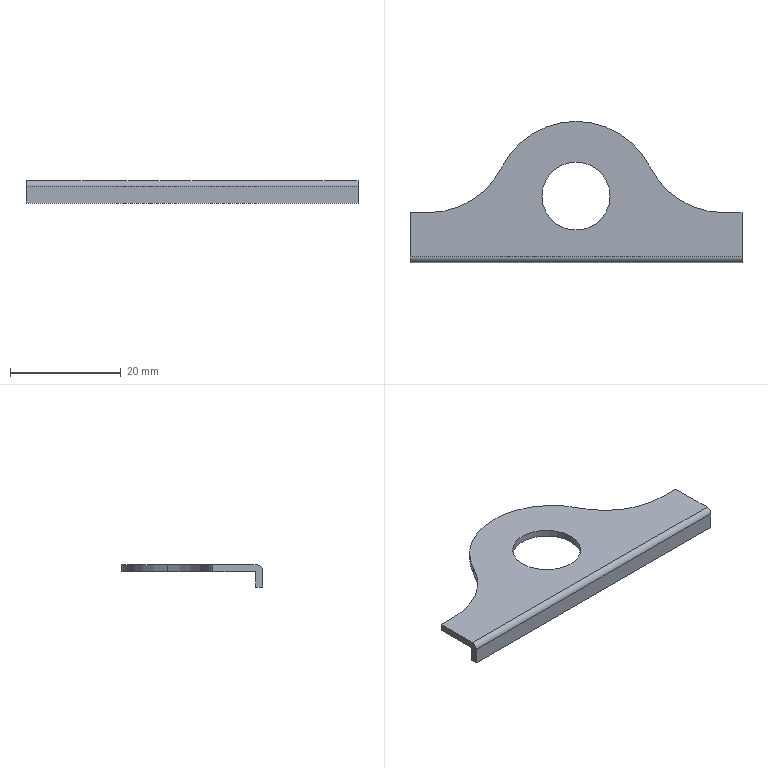Part | STEP file | gslz 2016.10.28-13_id962_x_t | 1 solid | 14 faces | box 60 x 25.5 x 4 mm | volume 1272 mm3 | plane 9 | cylinder 5 | commonest cylinder face diameters 30 x3 2 x1 12.3 x1
STEP:
#1=CARTESIAN_POINT('',(0.,0.,0.));
#2=DIRECTION('',(0.,0.,1.));
#3=DIRECTION('',(1.,0.,0.));
#4=AXIS2_PLACEMENT_3D('',#1,#2,#3);
#5=CARTESIAN_POINT('',(-668.704,-254.,1.25));
#6=VERTEX_POINT('',#5);
#7=CARTESIAN_POINT('',(-662.554,-254.,1.25));
#8=DIRECTION('',(0.,0.,1.));
#9=DIRECTION('',(-1.,0.,0.));
#10=AXIS2_PLACEMENT_3D('',#7,#8,#9);
#11=CIRCLE('',#10,6.15);
#12=CARTESIAN_POINT('',(1793.591,319.067,1.25));
#13=DIRECTION('',(0.,0.,1.));
#14=DIRECTION('',(1.,0.,0.));
#15=AXIS2_PLACEMENT_3D('',#12,#13,#14);
#16=PLANE('',#15);
#17=CARTESIAN_POINT('',(-2456.145,-573.067));
#18=DIRECTION('',(-1.,0.));
#19=AXIS2_PLACEMENT_2D('',#17,#18);
#20=CIRCLE('',#19,6.15);
#21=(GEOMETRIC_REPRESENTATION_CONTEXT(2)PARAMETRIC_REPRESENTATION_CONTEXT()REPRESENTATION_CONTEXT('',''));
#22=DEFINITIONAL_REPRESENTATION('',(#20),#21);
#23=PCURVE('',#16,#22);
#24=CARTESIAN_POINT('',(-662.554,-254.,2.5));
#25=DIRECTION('',(0.,0.,-1.));
#26=DIRECTION('',(1.,0.,0.));
#27=AXIS2_PLACEMENT_3D('',#24,#25,#26);
#28=CYLINDRICAL_SURFACE('',#27,6.15);
#29=CARTESIAN_POINT('',(9.425,1.25));
#30=DIRECTION('',(-1.,0.));
#31=VECTOR('',#30,1.);
#32=LINE('',#29,#31);
#33=(GEOMETRIC_REPRESENTATION_CONTEXT(2)PARAMETRIC_REPRESENTATION_CONTEXT()REPRESENTATION_CONTEXT('',''));
#34=DEFINITIONAL_REPRESENTATION('',(#32),#33);
#35=PCURVE('',#28,#34);
#36=SURFACE_CURVE('',#11,(#23,#35),.PCURVE_S1.);
#37=EDGE_CURVE('',#6,#6,#36,.T.);
#38=ORIENTED_EDGE('',*,*,#37,.F.);
#39=EDGE_LOOP('',(#38));
#40=FACE_BOUND('',#39,.T.);
#41=CARTESIAN_POINT('',(-692.554,-257.,1.25));
#42=VERTEX_POINT('',#41);
#43=CARTESIAN_POINT('',(-689.345,-257.,1.25));
#44=VERTEX_POINT('',#43);
#45=CARTESIAN_POINT('',(1793.591,-257.,1.25));
#46=DIRECTION('',(1.,0.,0.));
#47=VECTOR('',#46,1.);
#48=LINE('',#45,#47);
#49=CARTESIAN_POINT('',(0.,-576.067));
#50=DIRECTION('',(1.,0.));
#51=VECTOR('',#50,1.);
#52=LINE('',#49,#51);
#53=(GEOMETRIC_REPRESENTATION_CONTEXT(2)PARAMETRIC_REPRESENTATION_CONTEXT()REPRESENTATION_CONTEXT('',''));
#54=DEFINITIONAL_REPRESENTATION('',(#52),#53);
#55=PCURVE('',#16,#54);
#56=CARTESIAN_POINT('',(-705.557,-257.,2.5));
#57=DIRECTION('',(0.,1.,0.));
#58=DIRECTION('',(0.,0.,1.));
#59=AXIS2_PLACEMENT_3D('',#56,#57,#58);
#60=PLANE('',#59);
#61=CARTESIAN_POINT('',(-1.25,2499.149));
#62=DIRECTION('',(0.,1.));
#63=VECTOR('',#62,1.);
#64=LINE('',#61,#63);
#65=(GEOMETRIC_REPRESENTATION_CONTEXT(2)PARAMETRIC_REPRESENTATION_CONTEXT()REPRESENTATION_CONTEXT('',''));
#66=DEFINITIONAL_REPRESENTATION('',(#64),#65);
#67=PCURVE('',#60,#66);
#68=SURFACE_CURVE('',#48,(#55,#67),.PCURVE_S1.);
#69=EDGE_CURVE('',#42,#44,#68,.T.);
#70=ORIENTED_EDGE('',*,*,#69,.F.);
#71=CARTESIAN_POINT('',(-692.554,-265.,1.25));
#72=VERTEX_POINT('',#71);
#73=CARTESIAN_POINT('',(-692.554,319.067,1.25));
#74=DIRECTION('',(0.,1.,0.));
#75=VECTOR('',#74,1.);
#76=LINE('',#73,#75);
#77=CARTESIAN_POINT('',(-2486.145,0.));
#78=DIRECTION('',(0.,1.));
#79=VECTOR('',#78,1.);
#80=LINE('',#77,#79);
#81=(GEOMETRIC_REPRESENTATION_CONTEXT(2)PARAMETRIC_REPRESENTATION_CONTEXT()REPRESENTATION_CONTEXT('',''));
#82=DEFINITIONAL_REPRESENTATION('',(#80),#81);
#83=PCURVE('',#16,#82);
#84=CARTESIAN_POINT('',(-692.554,-244.358,-2.25));
#85=DIRECTION('',(-1.,0.,0.));
#86=DIRECTION('',(0.,0.,1.));
#87=AXIS2_PLACEMENT_3D('',#84,#85,#86);
#88=PLANE('',#87);
#89=CARTESIAN_POINT('',(3.5,563.425));
#90=DIRECTION('',(0.,1.));
#91=VECTOR('',#90,1.);
#92=LINE('',#89,#91);
#93=(GEOMETRIC_REPRESENTATION_CONTEXT(2)PARAMETRIC_REPRESENTATION_CONTEXT()REPRESENTATION_CONTEXT('',''));
#94=DEFINITIONAL_REPRESENTATION('',(#92),#93);
#95=PCURVE('',#88,#94);
#96=SURFACE_CURVE('',#76,(#83,#95),.PCURVE_S1.);
#97=EDGE_CURVE('',#72,#42,#96,.T.);
#98=ORIENTED_EDGE('',*,*,#97,.F.);
#99=CARTESIAN_POINT('',(-632.554,-265.,1.25));
#100=VERTEX_POINT('',#99);
#101=CARTESIAN_POINT('',(1793.591,-265.,1.25));
#102=DIRECTION('',(1.,0.,0.));
#103=VECTOR('',#102,1.);
#104=LINE('',#101,#103);
#105=CARTESIAN_POINT('',(0.,-584.067));
#106=DIRECTION('',(1.,0.));
#107=VECTOR('',#106,1.);
#108=LINE('',#105,#107);
#109=(GEOMETRIC_REPRESENTATION_CONTEXT(2)PARAMETRIC_REPRESENTATION_CONTEXT()REPRESENTATION_CONTEXT('',''));
#110=DEFINITIONAL_REPRESENTATION('',(#108),#109);
#111=PCURVE('',#16,#110);
#112=CARTESIAN_POINT('',(1793.591,-265.,0.25));
#113=DIRECTION('',(1.,0.,0.));
#114=DIRECTION('',(0.,1.,0.));
#115=AXIS2_PLACEMENT_3D('',#112,#113,#114);
#116=CYLINDRICAL_SURFACE('',#115,1.);
#117=CARTESIAN_POINT('',(1.571,0.));
#118=DIRECTION('',(0.,1.));
#119=VECTOR('',#118,1.);
#120=LINE('',#117,#119);
#121=(GEOMETRIC_REPRESENTATION_CONTEXT(2)PARAMETRIC_REPRESENTATION_CONTEXT()REPRESENTATION_CONTEXT('',''));
#122=DEFINITIONAL_REPRESENTATION('',(#120),#121);
#123=PCURVE('',#116,#122);
#124=SURFACE_CURVE('',#104,(#111,#123),.PCURVE_S1.);
#125=EDGE_CURVE('',#72,#100,#124,.T.);
#126=ORIENTED_EDGE('',*,*,#125,.T.);
#127=CARTESIAN_POINT('',(-632.554,-257.,1.25));
#128=VERTEX_POINT('',#127);
#129=CARTESIAN_POINT('',(-632.554,319.067,1.25));
#130=DIRECTION('',(0.,1.,0.));
#131=VECTOR('',#130,1.);
#132=LINE('',#129,#131);
#133=CARTESIAN_POINT('',(-2426.145,0.));
#134=DIRECTION('',(0.,1.));
#135=VECTOR('',#134,1.);
#136=LINE('',#133,#135);
#137=(GEOMETRIC_REPRESENTATION_CONTEXT(2)PARAMETRIC_REPRESENTATION_CONTEXT()REPRESENTATION_CONTEXT('',''));
#138=DEFINITIONAL_REPRESENTATION('',(#136),#137);
#139=PCURVE('',#16,#138);
#140=CARTESIAN_POINT('',(-632.554,-244.358,-2.25));
#141=DIRECTION('',(1.,0.,0.));
#142=DIRECTION('',(0.,0.,-1.));
#143=AXIS2_PLACEMENT_3D('',#140,#141,#142);
#144=PLANE('',#143);
#145=CARTESIAN_POINT('',(-3.5,563.425));
#146=DIRECTION('',(0.,1.));
#147=VECTOR('',#146,1.);
#148=LINE('',#145,#147);
#149=(GEOMETRIC_REPRESENTATION_CONTEXT(2)PARAMETRIC_REPRESENTATION_CONTEXT()REPRESENTATION_CONTEXT('',''));
#150=DEFINITIONAL_REPRESENTATION('',(#148),#149);
#151=PCURVE('',#144,#150);
#152=SURFACE_CURVE('',#132,(#139,#151),.PCURVE_S1.);
#153=EDGE_CURVE('',#100,#128,#152,.T.);
#154=ORIENTED_EDGE('',*,*,#153,.T.);
#155=CARTESIAN_POINT('',(-635.763,-257.,1.25));
#156=VERTEX_POINT('',#155);
#157=CARTESIAN_POINT('',(-2874.517,-257.,1.25));
#158=DIRECTION('',(1.,0.,0.));
#159=VECTOR('',#158,1.);
#160=LINE('',#157,#159);
#161=CARTESIAN_POINT('',(-4668.108,-576.067));
#162=DIRECTION('',(1.,0.));
#163=VECTOR('',#162,1.);
#164=LINE('',#161,#163);
#165=(GEOMETRIC_REPRESENTATION_CONTEXT(2)PARAMETRIC_REPRESENTATION_CONTEXT()REPRESENTATION_CONTEXT('',''));
#166=DEFINITIONAL_REPRESENTATION('',(#164),#165);
#167=PCURVE('',#16,#166);
#168=CARTESIAN_POINT('',(-614.757,-257.,2.5));
#169=DIRECTION('',(0.,1.,0.));
#170=DIRECTION('',(-1.,0.,0.));
#171=AXIS2_PLACEMENT_3D('',#168,#169,#170);
#172=PLANE('',#171);
#173=CARTESIAN_POINT('',(2259.76,-1.25));
#174=DIRECTION('',(-1.,0.));
#175=VECTOR('',#174,1.);
#176=LINE('',#173,#175);
#177=(GEOMETRIC_REPRESENTATION_CONTEXT(2)PARAMETRIC_REPRESENTATION_CONTEXT()REPRESENTATION_CONTEXT('',''));
#178=DEFINITIONAL_REPRESENTATION('',(#176),#177);
#179=PCURVE('',#172,#178);
#180=SURFACE_CURVE('',#160,(#167,#179),.PCURVE_S1.);
#181=EDGE_CURVE('',#156,#128,#180,.T.);
#182=ORIENTED_EDGE('',*,*,#181,.F.);
#183=CARTESIAN_POINT('',(-649.158,-248.75,1.25));
#184=VERTEX_POINT('',#183);
#185=CARTESIAN_POINT('',(-635.763,-242.,1.25));
#186=DIRECTION('',(0.,0.,-1.));
#187=DIRECTION('',(-1.,0.,0.));
#188=AXIS2_PLACEMENT_3D('',#185,#186,#187);
#189=CIRCLE('',#188,15.);
#190=CARTESIAN_POINT('',(-2444.354,-561.067));
#191=CARTESIAN_POINT('',(-2444.354,-535.086));
#192=CARTESIAN_POINT('',(-2421.854,-548.076));
#193=CARTESIAN_POINT('',(-2399.354,-561.067));
#194=CARTESIAN_POINT('',(-2421.854,-574.057));
#195=CARTESIAN_POINT('',(-2444.354,-587.048));
#196=CARTESIAN_POINT('',(-2444.354,-561.067));
#197=(BOUNDED_CURVE()B_SPLINE_CURVE(2,(#190,#191,#192,#193,#194,#195,#196),.UNSPECIFIED.,.T.,.F.)B_SPLINE_CURVE_WITH_KNOTS((1,2,2,2,2,1),(-2.094,0.,2.094,4.189,6.283,8.378),.UNSPECIFIED.)CURVE()GEOMETRIC_REPRESENTATION_ITEM()RATIONAL_B_SPLINE_CURVE((1.,0.5,1.,0.5,1.,0.5,1.))REPRESENTATION_ITEM(''));
#198=(GEOMETRIC_REPRESENTATION_CONTEXT(2)PARAMETRIC_REPRESENTATION_CONTEXT()REPRESENTATION_CONTEXT('',''));
#199=DEFINITIONAL_REPRESENTATION('',(#197),#198);
#200=PCURVE('',#16,#199);
#201=CARTESIAN_POINT('',(-635.763,-242.,2.5));
#202=DIRECTION('',(0.,0.,-1.));
#203=DIRECTION('',(1.,0.,0.));
#204=AXIS2_PLACEMENT_3D('',#201,#202,#203);
#205=CYLINDRICAL_SURFACE('',#204,15.);
#206=CARTESIAN_POINT('',(-3.142,1.25));
#207=DIRECTION('',(1.,0.));
#208=VECTOR('',#207,1.);
#209=LINE('',#206,#208);
#210=(GEOMETRIC_REPRESENTATION_CONTEXT(2)PARAMETRIC_REPRESENTATION_CONTEXT()REPRESENTATION_CONTEXT('',''));
#211=DEFINITIONAL_REPRESENTATION('',(#209),#210);
#212=PCURVE('',#205,#211);
#213=SURFACE_CURVE('',#189,(#200,#212),.PCURVE_S1.);
#214=EDGE_CURVE('',#156,#184,#213,.T.);
#215=ORIENTED_EDGE('',*,*,#214,.T.);
#216=CARTESIAN_POINT('',(-675.949,-248.75,1.25));
#217=VERTEX_POINT('',#216);
#218=CARTESIAN_POINT('',(-662.554,-255.5,1.25));
#219=DIRECTION('',(0.,0.,1.));
#220=DIRECTION('',(-1.,0.,0.));
#221=AXIS2_PLACEMENT_3D('',#218,#219,#220);
#222=CIRCLE('',#221,15.);
#223=CARTESIAN_POINT('',(-2456.145,-574.567));
#224=DIRECTION('',(-1.,0.));
#225=AXIS2_PLACEMENT_2D('',#223,#224);
#226=CIRCLE('',#225,15.);
#227=(GEOMETRIC_REPRESENTATION_CONTEXT(2)PARAMETRIC_REPRESENTATION_CONTEXT()REPRESENTATION_CONTEXT('',''));
#228=DEFINITIONAL_REPRESENTATION('',(#226),#227);
#229=PCURVE('',#16,#228);
#230=CARTESIAN_POINT('',(-662.554,-255.5,2.5));
#231=DIRECTION('',(0.,0.,-1.));
#232=DIRECTION('',(1.,0.,0.));
#233=AXIS2_PLACEMENT_3D('',#230,#231,#232);
#234=CYLINDRICAL_SURFACE('',#233,15.);
#235=CARTESIAN_POINT('',(9.425,1.25));
#236=DIRECTION('',(-1.,0.));
#237=VECTOR('',#236,1.);
#238=LINE('',#235,#237);
#239=(GEOMETRIC_REPRESENTATION_CONTEXT(2)PARAMETRIC_REPRESENTATION_CONTEXT()REPRESENTATION_CONTEXT('',''));
#240=DEFINITIONAL_REPRESENTATION('',(#238),#239);
#241=PCURVE('',#234,#240);
#242=SURFACE_CURVE('',#222,(#229,#241),.PCURVE_S1.);
#243=EDGE_CURVE('',#184,#217,#242,.T.);
#244=ORIENTED_EDGE('',*,*,#243,.T.);
#245=CARTESIAN_POINT('',(-689.345,-242.,1.25));
#246=DIRECTION('',(0.,0.,-1.));
#247=DIRECTION('',(-1.,0.,0.));
#248=AXIS2_PLACEMENT_3D('',#245,#246,#247);
#249=CIRCLE('',#248,15.);
#250=CARTESIAN_POINT('',(-2497.936,-561.067));
#251=CARTESIAN_POINT('',(-2497.936,-535.086));
#252=CARTESIAN_POINT('',(-2475.436,-548.076));
#253=CARTESIAN_POINT('',(-2452.936,-561.067));
#254=CARTESIAN_POINT('',(-2475.436,-574.057));
#255=CARTESIAN_POINT('',(-2497.936,-587.048));
#256=CARTESIAN_POINT('',(-2497.936,-561.067));
#257=(BOUNDED_CURVE()B_SPLINE_CURVE(2,(#250,#251,#252,#253,#254,#255,#256),.UNSPECIFIED.,.T.,.F.)B_SPLINE_CURVE_WITH_KNOTS((1,2,2,2,2,1),(-2.094,0.,2.094,4.189,6.283,8.378),.UNSPECIFIED.)CURVE()GEOMETRIC_REPRESENTATION_ITEM()RATIONAL_B_SPLINE_CURVE((1.,0.5,1.,0.5,1.,0.5,1.))REPRESENTATION_ITEM(''));
#258=(GEOMETRIC_REPRESENTATION_CONTEXT(2)PARAMETRIC_REPRESENTATION_CONTEXT()REPRESENTATION_CONTEXT('',''));
#259=DEFINITIONAL_REPRESENTATION('',(#257),#258);
#260=PCURVE('',#16,#259);
#261=CARTESIAN_POINT('',(-689.345,-242.,2.5));
#262=DIRECTION('',(0.,0.,-1.));
#263=DIRECTION('',(1.,0.,0.));
#264=AXIS2_PLACEMENT_3D('',#261,#262,#263);
#265=CYLINDRICAL_SURFACE('',#264,15.);
#266=CARTESIAN_POINT('',(-3.142,1.25));
#267=DIRECTION('',(1.,0.));
#268=VECTOR('',#267,1.);
#269=LINE('',#266,#268);
#270=(GEOMETRIC_REPRESENTATION_CONTEXT(2)PARAMETRIC_REPRESENTATION_CONTEXT()REPRESENTATION_CONTEXT('',''));
#271=DEFINITIONAL_REPRESENTATION('',(#269),#270);
#272=PCURVE('',#265,#271);
#273=SURFACE_CURVE('',#249,(#260,#272),.PCURVE_S1.);
#274=EDGE_CURVE('',#217,#44,#273,.T.);
#275=ORIENTED_EDGE('',*,*,#274,.T.);
#276=EDGE_LOOP('',(#70,#98,#126,#154,#182,#215,#244,#275));
#277=FACE_BOUND('',#276,.T.);
#278=ADVANCED_FACE('',(#40,#277),#16,.T.);
#279=CARTESIAN_POINT('',(-668.704,-254.,0.));
#280=VERTEX_POINT('',#279);
#281=CARTESIAN_POINT('',(-662.554,-254.,0.));
#282=DIRECTION('',(0.,0.,-1.));
#283=DIRECTION('',(-1.,0.,0.));
#284=AXIS2_PLACEMENT_3D('',#281,#282,#283);
#285=CIRCLE('',#284,6.15);
#286=CARTESIAN_POINT('',(1793.591,319.067,0.));
#287=DIRECTION('',(0.,0.,1.));
#288=DIRECTION('',(1.,0.,0.));
#289=AXIS2_PLACEMENT_3D('',#286,#287,#288);
#290=PLANE('',#289);
#291=CARTESIAN_POINT('',(-2462.295,-573.067));
#292=CARTESIAN_POINT('',(-2462.295,-562.415));
#293=CARTESIAN_POINT('',(-2453.07,-567.741));
#294=CARTESIAN_POINT('',(-2443.845,-573.067));
#295=CARTESIAN_POINT('',(-2453.07,-578.393));
#296=CARTESIAN_POINT('',(-2462.295,-583.719));
#297=CARTESIAN_POINT('',(-2462.295,-573.067));
#298=(BOUNDED_CURVE()B_SPLINE_CURVE(2,(#291,#292,#293,#294,#295,#296,#297),.UNSPECIFIED.,.T.,.F.)B_SPLINE_CURVE_WITH_KNOTS((1,2,2,2,2,1),(-2.094,0.,2.094,4.189,6.283,8.378),.UNSPECIFIED.)CURVE()GEOMETRIC_REPRESENTATION_ITEM()RATIONAL_B_SPLINE_CURVE((1.,0.5,1.,0.5,1.,0.5,1.))REPRESENTATION_ITEM(''));
#299=(GEOMETRIC_REPRESENTATION_CONTEXT(2)PARAMETRIC_REPRESENTATION_CONTEXT()REPRESENTATION_CONTEXT('',''));
#300=DEFINITIONAL_REPRESENTATION('',(#298),#299);
#301=PCURVE('',#290,#300);
#302=CARTESIAN_POINT('',(3.142,2.5));
#303=DIRECTION('',(1.,0.));
#304=VECTOR('',#303,1.);
#305=LINE('',#302,#304);
#306=(GEOMETRIC_REPRESENTATION_CONTEXT(2)PARAMETRIC_REPRESENTATION_CONTEXT()REPRESENTATION_CONTEXT('',''));
#307=DEFINITIONAL_REPRESENTATION('',(#305),#306);
#308=PCURVE('',#28,#307);
#309=SURFACE_CURVE('',#285,(#301,#308),.PCURVE_S1.);
#310=EDGE_CURVE('',#280,#280,#309,.T.);
#311=ORIENTED_EDGE('',*,*,#310,.F.);
#312=EDGE_LOOP('',(#311));
#313=FACE_BOUND('',#312,.T.);
#314=CARTESIAN_POINT('',(-692.554,-257.,0.));
#315=VERTEX_POINT('',#314);
#316=CARTESIAN_POINT('',(-692.554,-264.75,0.));
#317=VERTEX_POINT('',#316);
#318=CARTESIAN_POINT('',(-692.554,319.067,0.));
#319=DIRECTION('',(0.,-1.,0.));
#320=VECTOR('',#319,1.);
#321=LINE('',#318,#320);
#322=CARTESIAN_POINT('',(-2486.145,0.));
#323=DIRECTION('',(0.,-1.));
#324=VECTOR('',#323,1.);
#325=LINE('',#322,#324);
#326=(GEOMETRIC_REPRESENTATION_CONTEXT(2)PARAMETRIC_REPRESENTATION_CONTEXT()REPRESENTATION_CONTEXT('',''));
#327=DEFINITIONAL_REPRESENTATION('',(#325),#326);
#328=PCURVE('',#290,#327);
#329=CARTESIAN_POINT('',(2.25,563.425));
#330=DIRECTION('',(0.,-1.));
#331=VECTOR('',#330,1.);
#332=LINE('',#329,#331);
#333=(GEOMETRIC_REPRESENTATION_CONTEXT(2)PARAMETRIC_REPRESENTATION_CONTEXT()REPRESENTATION_CONTEXT('',''));
#334=DEFINITIONAL_REPRESENTATION('',(#332),#333);
#335=PCURVE('',#88,#334);
#336=SURFACE_CURVE('',#321,(#328,#335),.PCURVE_S1.);
#337=EDGE_CURVE('',#315,#317,#336,.T.);
#338=ORIENTED_EDGE('',*,*,#337,.F.);
#339=CARTESIAN_POINT('',(-689.345,-257.,0.));
#340=VERTEX_POINT('',#339);
#341=CARTESIAN_POINT('',(-705.557,-257.,0.));
#342=DIRECTION('',(1.,0.,0.));
#343=VECTOR('',#342,1.);
#344=LINE('',#341,#343);
#345=CARTESIAN_POINT('',(-2499.149,-576.067));
#346=DIRECTION('',(1.,0.));
#347=VECTOR('',#346,1.);
#348=LINE('',#345,#347);
#349=(GEOMETRIC_REPRESENTATION_CONTEXT(2)PARAMETRIC_REPRESENTATION_CONTEXT()REPRESENTATION_CONTEXT('',''));
#350=DEFINITIONAL_REPRESENTATION('',(#348),#349);
#351=PCURVE('',#290,#350);
#352=CARTESIAN_POINT('',(-2.5,0.));
#353=DIRECTION('',(0.,1.));
#354=VECTOR('',#353,1.);
#355=LINE('',#352,#354);
#356=(GEOMETRIC_REPRESENTATION_CONTEXT(2)PARAMETRIC_REPRESENTATION_CONTEXT()REPRESENTATION_CONTEXT('',''));
#357=DEFINITIONAL_REPRESENTATION('',(#355),#356);
#358=PCURVE('',#60,#357);
#359=SURFACE_CURVE('',#344,(#351,#358),.PCURVE_S1.);
#360=EDGE_CURVE('',#315,#340,#359,.T.);
#361=ORIENTED_EDGE('',*,*,#360,.T.);
#362=CARTESIAN_POINT('',(-675.949,-248.75,0.));
#363=VERTEX_POINT('',#362);
#364=CARTESIAN_POINT('',(-689.345,-242.,0.));
#365=DIRECTION('',(0.,0.,1.));
#366=DIRECTION('',(-1.,0.,0.));
#367=AXIS2_PLACEMENT_3D('',#364,#365,#366);
#368=CIRCLE('',#367,15.);
#369=CARTESIAN_POINT('',(-2482.936,-561.067));
#370=DIRECTION('',(-1.,0.));
#371=AXIS2_PLACEMENT_2D('',#369,#370);
#372=CIRCLE('',#371,15.);
#373=(GEOMETRIC_REPRESENTATION_CONTEXT(2)PARAMETRIC_REPRESENTATION_CONTEXT()REPRESENTATION_CONTEXT('',''));
#374=DEFINITIONAL_REPRESENTATION('',(#372),#373);
#375=PCURVE('',#290,#374);
#376=CARTESIAN_POINT('',(3.142,2.5));
#377=DIRECTION('',(-1.,0.));
#378=VECTOR('',#377,1.);
#379=LINE('',#376,#378);
#380=(GEOMETRIC_REPRESENTATION_CONTEXT(2)PARAMETRIC_REPRESENTATION_CONTEXT()REPRESENTATION_CONTEXT('',''));
#381=DEFINITIONAL_REPRESENTATION('',(#379),#380);
#382=PCURVE('',#265,#381);
#383=SURFACE_CURVE('',#368,(#375,#382),.PCURVE_S1.);
#384=EDGE_CURVE('',#340,#363,#383,.T.);
#385=ORIENTED_EDGE('',*,*,#384,.T.);
#386=CARTESIAN_POINT('',(-649.158,-248.75,0.));
#387=VERTEX_POINT('',#386);
#388=CARTESIAN_POINT('',(-662.554,-255.5,0.));
#389=DIRECTION('',(0.,0.,-1.));
#390=DIRECTION('',(-1.,0.,0.));
#391=AXIS2_PLACEMENT_3D('',#388,#389,#390);
#392=CIRCLE('',#391,15.);
#393=CARTESIAN_POINT('',(-2471.145,-574.567));
#394=CARTESIAN_POINT('',(-2471.145,-548.586));
#395=CARTESIAN_POINT('',(-2448.645,-561.576));
#396=CARTESIAN_POINT('',(-2426.145,-574.567));
#397=CARTESIAN_POINT('',(-2448.645,-587.557));
#398=CARTESIAN_POINT('',(-2471.145,-600.548));
#399=CARTESIAN_POINT('',(-2471.145,-574.567));
#400=(BOUNDED_CURVE()B_SPLINE_CURVE(2,(#393,#394,#395,#396,#397,#398,#399),.UNSPECIFIED.,.T.,.F.)B_SPLINE_CURVE_WITH_KNOTS((1,2,2,2,2,1),(-2.094,0.,2.094,4.189,6.283,8.378),.UNSPECIFIED.)CURVE()GEOMETRIC_REPRESENTATION_ITEM()RATIONAL_B_SPLINE_CURVE((1.,0.5,1.,0.5,1.,0.5,1.))REPRESENTATION_ITEM(''));
#401=(GEOMETRIC_REPRESENTATION_CONTEXT(2)PARAMETRIC_REPRESENTATION_CONTEXT()REPRESENTATION_CONTEXT('',''));
#402=DEFINITIONAL_REPRESENTATION('',(#400),#401);
#403=PCURVE('',#290,#402);
#404=CARTESIAN_POINT('',(3.142,2.5));
#405=DIRECTION('',(1.,0.));
#406=VECTOR('',#405,1.);
#407=LINE('',#404,#406);
#408=(GEOMETRIC_REPRESENTATION_CONTEXT(2)PARAMETRIC_REPRESENTATION_CONTEXT()REPRESENTATION_CONTEXT('',''));
#409=DEFINITIONAL_REPRESENTATION('',(#407),#408);
#410=PCURVE('',#234,#409);
#411=SURFACE_CURVE('',#392,(#403,#410),.PCURVE_S1.);
#412=EDGE_CURVE('',#363,#387,#411,.T.);
#413=ORIENTED_EDGE('',*,*,#412,.T.);
#414=CARTESIAN_POINT('',(-635.763,-257.,0.));
#415=VERTEX_POINT('',#414);
#416=CARTESIAN_POINT('',(-635.763,-242.,0.));
#417=DIRECTION('',(0.,0.,1.));
#418=DIRECTION('',(-1.,0.,0.));
#419=AXIS2_PLACEMENT_3D('',#416,#417,#418);
#420=CIRCLE('',#419,15.);
#421=CARTESIAN_POINT('',(-2429.354,-561.067));
#422=DIRECTION('',(-1.,0.));
#423=AXIS2_PLACEMENT_2D('',#421,#422);
#424=CIRCLE('',#423,15.);
#425=(GEOMETRIC_REPRESENTATION_CONTEXT(2)PARAMETRIC_REPRESENTATION_CONTEXT()REPRESENTATION_CONTEXT('',''));
#426=DEFINITIONAL_REPRESENTATION('',(#424),#425);
#427=PCURVE('',#290,#426);
#428=CARTESIAN_POINT('',(3.142,2.5));
#429=DIRECTION('',(-1.,0.));
#430=VECTOR('',#429,1.);
#431=LINE('',#428,#430);
#432=(GEOMETRIC_REPRESENTATION_CONTEXT(2)PARAMETRIC_REPRESENTATION_CONTEXT()REPRESENTATION_CONTEXT('',''));
#433=DEFINITIONAL_REPRESENTATION('',(#431),#432);
#434=PCURVE('',#205,#433);
#435=SURFACE_CURVE('',#420,(#427,#434),.PCURVE_S1.);
#436=EDGE_CURVE('',#387,#415,#435,.T.);
#437=ORIENTED_EDGE('',*,*,#436,.T.);
#438=CARTESIAN_POINT('',(-632.554,-257.,0.));
#439=VERTEX_POINT('',#438);
#440=CARTESIAN_POINT('',(-614.757,-257.,0.));
#441=DIRECTION('',(1.,0.,0.));
#442=VECTOR('',#441,1.);
#443=LINE('',#440,#442);
#444=CARTESIAN_POINT('',(-2408.349,-576.067));
#445=DIRECTION('',(1.,0.));
#446=VECTOR('',#445,1.);
#447=LINE('',#444,#446);
#448=(GEOMETRIC_REPRESENTATION_CONTEXT(2)PARAMETRIC_REPRESENTATION_CONTEXT()REPRESENTATION_CONTEXT('',''));
#449=DEFINITIONAL_REPRESENTATION('',(#447),#448);
#450=PCURVE('',#290,#449);
#451=CARTESIAN_POINT('',(0.,-2.5));
#452=DIRECTION('',(-1.,0.));
#453=VECTOR('',#452,1.);
#454=LINE('',#451,#453);
#455=(GEOMETRIC_REPRESENTATION_CONTEXT(2)PARAMETRIC_REPRESENTATION_CONTEXT()REPRESENTATION_CONTEXT('',''));
#456=DEFINITIONAL_REPRESENTATION('',(#454),#455);
#457=PCURVE('',#172,#456);
#458=SURFACE_CURVE('',#443,(#450,#457),.PCURVE_S1.);
#459=EDGE_CURVE('',#415,#439,#458,.T.);
#460=ORIENTED_EDGE('',*,*,#459,.T.);
#461=CARTESIAN_POINT('',(-632.554,-264.75,0.));
#462=VERTEX_POINT('',#461);
#463=CARTESIAN_POINT('',(-632.554,319.067,0.));
#464=DIRECTION('',(0.,-1.,0.));
#465=VECTOR('',#464,1.);
#466=LINE('',#463,#465);
#467=CARTESIAN_POINT('',(-2426.145,0.));
#468=DIRECTION('',(0.,-1.));
#469=VECTOR('',#468,1.);
#470=LINE('',#467,#469);
#471=(GEOMETRIC_REPRESENTATION_CONTEXT(2)PARAMETRIC_REPRESENTATION_CONTEXT()REPRESENTATION_CONTEXT('',''));
#472=DEFINITIONAL_REPRESENTATION('',(#470),#471);
#473=PCURVE('',#290,#472);
#474=CARTESIAN_POINT('',(-2.25,563.425));
#475=DIRECTION('',(0.,-1.));
#476=VECTOR('',#475,1.);
#477=LINE('',#474,#476);
#478=(GEOMETRIC_REPRESENTATION_CONTEXT(2)PARAMETRIC_REPRESENTATION_CONTEXT()REPRESENTATION_CONTEXT('',''));
#479=DEFINITIONAL_REPRESENTATION('',(#477),#478);
#480=PCURVE('',#144,#479);
#481=SURFACE_CURVE('',#466,(#473,#480),.PCURVE_S1.);
#482=EDGE_CURVE('',#439,#462,#481,.T.);
#483=ORIENTED_EDGE('',*,*,#482,.T.);
#484=CARTESIAN_POINT('',(1793.591,-264.75,0.));
#485=DIRECTION('',(1.,0.,0.));
#486=VECTOR('',#485,1.);
#487=LINE('',#484,#486);
#488=CARTESIAN_POINT('',(0.,-583.817));
#489=DIRECTION('',(1.,0.));
#490=VECTOR('',#489,1.);
#491=LINE('',#488,#490);
#492=(GEOMETRIC_REPRESENTATION_CONTEXT(2)PARAMETRIC_REPRESENTATION_CONTEXT()REPRESENTATION_CONTEXT('',''));
#493=DEFINITIONAL_REPRESENTATION('',(#491),#492);
#494=PCURVE('',#290,#493);
#495=CARTESIAN_POINT('',(1463.925,-264.75,-135.834));
#496=DIRECTION('',(0.,-1.,0.));
#497=DIRECTION('',(1.,0.,0.));
#498=AXIS2_PLACEMENT_3D('',#495,#496,#497);
#499=PLANE('',#498);
#500=CARTESIAN_POINT('',(329.666,135.834));
#501=DIRECTION('',(1.,0.));
#502=VECTOR('',#501,1.);
#503=LINE('',#500,#502);
#504=(GEOMETRIC_REPRESENTATION_CONTEXT(2)PARAMETRIC_REPRESENTATION_CONTEXT()REPRESENTATION_CONTEXT('',''));
#505=DEFINITIONAL_REPRESENTATION('',(#503),#504);
#506=PCURVE('',#499,#505);
#507=SURFACE_CURVE('',#487,(#494,#506),.PCURVE_S1.);
#508=EDGE_CURVE('',#317,#462,#507,.T.);
#509=ORIENTED_EDGE('',*,*,#508,.F.);
#510=EDGE_LOOP('',(#338,#361,#385,#413,#437,#460,#483,#509));
#511=FACE_BOUND('',#510,.T.);
#512=ADVANCED_FACE('',(#313,#511),#290,.F.);
#513=CARTESIAN_POINT('',(-692.554,-264.75,-2.75));
#514=VERTEX_POINT('',#513);
#515=CARTESIAN_POINT('',(-692.554,-264.75,-135.834));
#516=DIRECTION('',(0.,0.,1.));
#517=VECTOR('',#516,1.);
#518=LINE('',#515,#517);
#519=CARTESIAN_POINT('',(-2156.479,0.));
#520=DIRECTION('',(0.,1.));
#521=VECTOR('',#520,1.);
#522=LINE('',#519,#521);
#523=(GEOMETRIC_REPRESENTATION_CONTEXT(2)PARAMETRIC_REPRESENTATION_CONTEXT()REPRESENTATION_CONTEXT('',''));
#524=DEFINITIONAL_REPRESENTATION('',(#522),#523);
#525=PCURVE('',#499,#524);
#526=CARTESIAN_POINT('',(-133.584,-20.392));
#527=DIRECTION('',(1.,0.));
#528=VECTOR('',#527,1.);
#529=LINE('',#526,#528);
#530=(GEOMETRIC_REPRESENTATION_CONTEXT(2)PARAMETRIC_REPRESENTATION_CONTEXT()REPRESENTATION_CONTEXT('',''));
#531=DEFINITIONAL_REPRESENTATION('',(#529),#530);
#532=PCURVE('',#88,#531);
#533=SURFACE_CURVE('',#518,(#525,#532),.PCURVE_S1.);
#534=EDGE_CURVE('',#514,#317,#533,.T.);
#535=ORIENTED_EDGE('',*,*,#534,.T.);
#536=ORIENTED_EDGE('',*,*,#508,.T.);
#537=CARTESIAN_POINT('',(-632.554,-264.75,-2.75));
#538=VERTEX_POINT('',#537);
#539=CARTESIAN_POINT('',(-632.554,-264.75,-135.834));
#540=DIRECTION('',(0.,0.,-1.));
#541=VECTOR('',#540,1.);
#542=LINE('',#539,#541);
#543=CARTESIAN_POINT('',(-2096.479,0.));
#544=DIRECTION('',(0.,-1.));
#545=VECTOR('',#544,1.);
#546=LINE('',#543,#545);
#547=(GEOMETRIC_REPRESENTATION_CONTEXT(2)PARAMETRIC_REPRESENTATION_CONTEXT()REPRESENTATION_CONTEXT('',''));
#548=DEFINITIONAL_REPRESENTATION('',(#546),#547);
#549=PCURVE('',#499,#548);
#550=CARTESIAN_POINT('',(133.584,-20.392));
#551=DIRECTION('',(1.,0.));
#552=VECTOR('',#551,1.);
#553=LINE('',#550,#552);
#554=(GEOMETRIC_REPRESENTATION_CONTEXT(2)PARAMETRIC_REPRESENTATION_CONTEXT()REPRESENTATION_CONTEXT('',''));
#555=DEFINITIONAL_REPRESENTATION('',(#553),#554);
#556=PCURVE('',#144,#555);
#557=SURFACE_CURVE('',#542,(#549,#556),.PCURVE_S1.);
#558=EDGE_CURVE('',#462,#538,#557,.T.);
#559=ORIENTED_EDGE('',*,*,#558,.T.);
#560=CARTESIAN_POINT('',(-1810.,-264.75,-2.75));
#561=DIRECTION('',(-1.,0.,0.));
#562=VECTOR('',#561,1.);
#563=LINE('',#560,#562);
#564=CARTESIAN_POINT('',(-3273.925,133.084));
#565=DIRECTION('',(-1.,0.));
#566=VECTOR('',#565,1.);
#567=LINE('',#564,#566);
#568=(GEOMETRIC_REPRESENTATION_CONTEXT(2)PARAMETRIC_REPRESENTATION_CONTEXT()REPRESENTATION_CONTEXT('',''));
#569=DEFINITIONAL_REPRESENTATION('',(#567),#568);
#570=PCURVE('',#499,#569);
#571=CARTESIAN_POINT('',(-1810.,-266.,-2.75));
#572=DIRECTION('',(0.,0.,1.));
#573=DIRECTION('',(-1.,0.,0.));
#574=AXIS2_PLACEMENT_3D('',#571,#572,#573);
#575=PLANE('',#574);
#576=CARTESIAN_POINT('',(0.,-1.25));
#577=DIRECTION('',(1.,0.));
#578=VECTOR('',#577,1.);
#579=LINE('',#576,#578);
#580=(GEOMETRIC_REPRESENTATION_CONTEXT(2)PARAMETRIC_REPRESENTATION_CONTEXT()REPRESENTATION_CONTEXT('',''));
#581=DEFINITIONAL_REPRESENTATION('',(#579),#580);
#582=PCURVE('',#575,#581);
#583=SURFACE_CURVE('',#563,(#570,#582),.PCURVE_S1.);
#584=EDGE_CURVE('',#538,#514,#583,.T.);
#585=ORIENTED_EDGE('',*,*,#584,.T.);
#586=EDGE_LOOP('',(#535,#536,#559,#585));
#587=FACE_BOUND('',#586,.T.);
#588=ADVANCED_FACE('',(#587),#499,.F.);
#589=CARTESIAN_POINT('',(-692.554,-266.,-2.75));
#590=VERTEX_POINT('',#589);
#591=CARTESIAN_POINT('',(-692.554,-266.,-2.75));
#592=DIRECTION('',(0.,1.,0.));
#593=VECTOR('',#592,1.);
#594=LINE('',#591,#593);
#595=CARTESIAN_POINT('',(-1117.446,0.));
#596=DIRECTION('',(0.,-1.));
#597=VECTOR('',#596,1.);
#598=LINE('',#595,#597);
#599=(GEOMETRIC_REPRESENTATION_CONTEXT(2)PARAMETRIC_REPRESENTATION_CONTEXT()REPRESENTATION_CONTEXT('',''));
#600=DEFINITIONAL_REPRESENTATION('',(#598),#599);
#601=PCURVE('',#575,#600);
#602=CARTESIAN_POINT('',(-0.5,-21.642));
#603=DIRECTION('',(0.,1.));
#604=VECTOR('',#603,1.);
#605=LINE('',#602,#604);
#606=(GEOMETRIC_REPRESENTATION_CONTEXT(2)PARAMETRIC_REPRESENTATION_CONTEXT()REPRESENTATION_CONTEXT('',''));
#607=DEFINITIONAL_REPRESENTATION('',(#605),#606);
#608=PCURVE('',#88,#607);
#609=SURFACE_CURVE('',#594,(#601,#608),.PCURVE_S1.);
#610=EDGE_CURVE('',#590,#514,#609,.T.);
#611=ORIENTED_EDGE('',*,*,#610,.T.);
#612=ORIENTED_EDGE('',*,*,#584,.F.);
#613=CARTESIAN_POINT('',(-632.554,-266.,-2.75));
#614=VERTEX_POINT('',#613);
#615=CARTESIAN_POINT('',(-632.554,-266.,-2.75));
#616=DIRECTION('',(0.,1.,0.));
#617=VECTOR('',#616,1.);
#618=LINE('',#615,#617);
#619=CARTESIAN_POINT('',(-1177.446,0.));
#620=DIRECTION('',(0.,-1.));
#621=VECTOR('',#620,1.);
#622=LINE('',#619,#621);
#623=(GEOMETRIC_REPRESENTATION_CONTEXT(2)PARAMETRIC_REPRESENTATION_CONTEXT()REPRESENTATION_CONTEXT('',''));
#624=DEFINITIONAL_REPRESENTATION('',(#622),#623);
#625=PCURVE('',#575,#624);
#626=CARTESIAN_POINT('',(0.5,-21.642));
#627=DIRECTION('',(0.,1.));
#628=VECTOR('',#627,1.);
#629=LINE('',#626,#628);
#630=(GEOMETRIC_REPRESENTATION_CONTEXT(2)PARAMETRIC_REPRESENTATION_CONTEXT()REPRESENTATION_CONTEXT('',''));
#631=DEFINITIONAL_REPRESENTATION('',(#629),#630);
#632=PCURVE('',#144,#631);
#633=SURFACE_CURVE('',#618,(#625,#632),.PCURVE_S1.);
#634=EDGE_CURVE('',#614,#538,#633,.T.);
#635=ORIENTED_EDGE('',*,*,#634,.F.);
#636=CARTESIAN_POINT('',(-1810.,-266.,-2.75));
#637=DIRECTION('',(-1.,0.,0.));
#638=VECTOR('',#637,1.);
#639=LINE('',#636,#638);
#640=CARTESIAN_POINT('',(0.,0.));
#641=DIRECTION('',(1.,0.));
#642=VECTOR('',#641,1.);
#643=LINE('',#640,#642);
#644=(GEOMETRIC_REPRESENTATION_CONTEXT(2)PARAMETRIC_REPRESENTATION_CONTEXT()REPRESENTATION_CONTEXT('',''));
#645=DEFINITIONAL_REPRESENTATION('',(#643),#644);
#646=PCURVE('',#575,#645);
#647=CARTESIAN_POINT('',(-548.575,-266.,0.625));
#648=DIRECTION('',(0.,-1.,0.));
#649=DIRECTION('',(1.,0.,0.));
#650=AXIS2_PLACEMENT_3D('',#647,#648,#649);
#651=PLANE('',#650);
#652=CARTESIAN_POINT('',(-1261.425,-3.375));
#653=DIRECTION('',(-1.,0.));
#654=VECTOR('',#653,1.);
#655=LINE('',#652,#654);
#656=(GEOMETRIC_REPRESENTATION_CONTEXT(2)PARAMETRIC_REPRESENTATION_CONTEXT()REPRESENTATION_CONTEXT('',''));
#657=DEFINITIONAL_REPRESENTATION('',(#655),#656);
#658=PCURVE('',#651,#657);
#659=SURFACE_CURVE('',#639,(#646,#658),.PCURVE_S1.);
#660=EDGE_CURVE('',#614,#590,#659,.T.);
#661=ORIENTED_EDGE('',*,*,#660,.T.);
#662=EDGE_LOOP('',(#611,#612,#635,#661));
#663=FACE_BOUND('',#662,.T.);
#664=ADVANCED_FACE('',(#663),#575,.F.);
#665=CARTESIAN_POINT('',(-632.554,-266.,0.25));
#666=VERTEX_POINT('',#665);
#667=CARTESIAN_POINT('',(-692.554,-266.,0.25));
#668=VERTEX_POINT('',#667);
#669=CARTESIAN_POINT('',(-548.575,-266.,0.25));
#670=DIRECTION('',(-1.,0.,0.));
#671=VECTOR('',#670,1.);
#672=LINE('',#669,#671);
#673=CARTESIAN_POINT('',(0.,-0.375));
#674=DIRECTION('',(-1.,0.));
#675=VECTOR('',#674,1.);
#676=LINE('',#673,#675);
#677=(GEOMETRIC_REPRESENTATION_CONTEXT(2)PARAMETRIC_REPRESENTATION_CONTEXT()REPRESENTATION_CONTEXT('',''));
#678=DEFINITIONAL_REPRESENTATION('',(#676),#677);
#679=PCURVE('',#651,#678);
#680=CARTESIAN_POINT('',(3.142,-2342.166));
#681=DIRECTION('',(0.,-1.));
#682=VECTOR('',#681,1.);
#683=LINE('',#680,#682);
#684=(GEOMETRIC_REPRESENTATION_CONTEXT(2)PARAMETRIC_REPRESENTATION_CONTEXT()REPRESENTATION_CONTEXT('',''));
#685=DEFINITIONAL_REPRESENTATION('',(#683),#684);
#686=PCURVE('',#116,#685);
#687=SURFACE_CURVE('',#672,(#679,#686),.PCURVE_S1.);
#688=EDGE_CURVE('',#666,#668,#687,.T.);
#689=ORIENTED_EDGE('',*,*,#688,.T.);
#690=CARTESIAN_POINT('',(-692.554,-266.,0.625));
#691=DIRECTION('',(0.,0.,-1.));
#692=VECTOR('',#691,1.);
#693=LINE('',#690,#692);
#694=CARTESIAN_POINT('',(-143.979,0.));
#695=DIRECTION('',(0.,-1.));
#696=VECTOR('',#695,1.);
#697=LINE('',#694,#696);
#698=(GEOMETRIC_REPRESENTATION_CONTEXT(2)PARAMETRIC_REPRESENTATION_CONTEXT()REPRESENTATION_CONTEXT('',''));
#699=DEFINITIONAL_REPRESENTATION('',(#697),#698);
#700=PCURVE('',#651,#699);
#701=CARTESIAN_POINT('',(2.875,-21.642));
#702=DIRECTION('',(-1.,0.));
#703=VECTOR('',#702,1.);
#704=LINE('',#701,#703);
#705=(GEOMETRIC_REPRESENTATION_CONTEXT(2)PARAMETRIC_REPRESENTATION_CONTEXT()REPRESENTATION_CONTEXT('',''));
#706=DEFINITIONAL_REPRESENTATION('',(#704),#705);
#707=PCURVE('',#88,#706);
#708=SURFACE_CURVE('',#693,(#700,#707),.PCURVE_S1.);
#709=EDGE_CURVE('',#668,#590,#708,.T.);
#710=ORIENTED_EDGE('',*,*,#709,.T.);
#711=ORIENTED_EDGE('',*,*,#660,.F.);
#712=CARTESIAN_POINT('',(-632.554,-266.,0.625));
#713=DIRECTION('',(0.,0.,-1.));
#714=VECTOR('',#713,1.);
#715=LINE('',#712,#714);
#716=CARTESIAN_POINT('',(-83.979,0.));
#717=DIRECTION('',(0.,-1.));
#718=VECTOR('',#717,1.);
#719=LINE('',#716,#718);
#720=(GEOMETRIC_REPRESENTATION_CONTEXT(2)PARAMETRIC_REPRESENTATION_CONTEXT()REPRESENTATION_CONTEXT('',''));
#721=DEFINITIONAL_REPRESENTATION('',(#719),#720);
#722=PCURVE('',#651,#721);
#723=CARTESIAN_POINT('',(-2.875,-21.642));
#724=DIRECTION('',(1.,0.));
#725=VECTOR('',#724,1.);
#726=LINE('',#723,#725);
#727=(GEOMETRIC_REPRESENTATION_CONTEXT(2)PARAMETRIC_REPRESENTATION_CONTEXT()REPRESENTATION_CONTEXT('',''));
#728=DEFINITIONAL_REPRESENTATION('',(#726),#727);
#729=PCURVE('',#144,#728);
#730=SURFACE_CURVE('',#715,(#722,#729),.PCURVE_S1.);
#731=EDGE_CURVE('',#666,#614,#730,.T.);
#732=ORIENTED_EDGE('',*,*,#731,.F.);
#733=EDGE_LOOP('',(#689,#710,#711,#732));
#734=FACE_BOUND('',#733,.T.);
#735=ADVANCED_FACE('',(#734),#651,.T.);
#736=ORIENTED_EDGE('',*,*,#125,.F.);
#737=CARTESIAN_POINT('',(-692.554,-265.,0.25));
#738=DIRECTION('',(1.,0.,0.));
#739=DIRECTION('',(0.,0.,1.));
#740=AXIS2_PLACEMENT_3D('',#737,#738,#739);
#741=CIRCLE('',#740,1.);
#742=CARTESIAN_POINT('',(1.571,-2486.145));
#743=DIRECTION('',(1.,0.));
#744=VECTOR('',#743,1.);
#745=LINE('',#742,#744);
#746=(GEOMETRIC_REPRESENTATION_CONTEXT(2)PARAMETRIC_REPRESENTATION_CONTEXT()REPRESENTATION_CONTEXT('',''));
#747=DEFINITIONAL_REPRESENTATION('',(#745),#746);
#748=PCURVE('',#116,#747);
#749=CARTESIAN_POINT('',(3.5,-20.642));
#750=CARTESIAN_POINT('',(3.5,-22.374));
#751=CARTESIAN_POINT('',(2.,-21.508));
#752=CARTESIAN_POINT('',(0.5,-20.642));
#753=CARTESIAN_POINT('',(2.,-19.776));
#754=CARTESIAN_POINT('',(3.5,-18.91));
#755=CARTESIAN_POINT('',(3.5,-20.642));
#756=(BOUNDED_CURVE()B_SPLINE_CURVE(2,(#749,#750,#751,#752,#753,#754,#755),.UNSPECIFIED.,.T.,.F.)B_SPLINE_CURVE_WITH_KNOTS((1,2,2,2,2,1),(-2.094,0.,2.094,4.189,6.283,8.378),.UNSPECIFIED.)CURVE()GEOMETRIC_REPRESENTATION_ITEM()RATIONAL_B_SPLINE_CURVE((1.,0.5,1.,0.5,1.,0.5,1.))REPRESENTATION_ITEM(''));
#757=(GEOMETRIC_REPRESENTATION_CONTEXT(2)PARAMETRIC_REPRESENTATION_CONTEXT()REPRESENTATION_CONTEXT('',''));
#758=DEFINITIONAL_REPRESENTATION('',(#756),#757);
#759=PCURVE('',#88,#758);
#760=SURFACE_CURVE('',#741,(#748,#759),.PCURVE_S1.);
#761=EDGE_CURVE('',#72,#668,#760,.T.);
#762=ORIENTED_EDGE('',*,*,#761,.T.);
#763=ORIENTED_EDGE('',*,*,#688,.F.);
#764=CARTESIAN_POINT('',(-632.554,-265.,0.25));
#765=DIRECTION('',(-1.,0.,0.));
#766=DIRECTION('',(0.,0.,-1.));
#767=AXIS2_PLACEMENT_3D('',#764,#765,#766);
#768=CIRCLE('',#767,1.);
#769=CARTESIAN_POINT('',(4.712,-2426.145));
#770=DIRECTION('',(-1.,0.));
#771=VECTOR('',#770,1.);
#772=LINE('',#769,#771);
#773=(GEOMETRIC_REPRESENTATION_CONTEXT(2)PARAMETRIC_REPRESENTATION_CONTEXT()REPRESENTATION_CONTEXT('',''));
#774=DEFINITIONAL_REPRESENTATION('',(#772),#773);
#775=PCURVE('',#116,#774);
#776=CARTESIAN_POINT('',(-1.5,-20.642));
#777=CARTESIAN_POINT('',(-1.5,-22.374));
#778=CARTESIAN_POINT('',(-3.,-21.508));
#779=CARTESIAN_POINT('',(-4.5,-20.642));
#780=CARTESIAN_POINT('',(-3.,-19.776));
#781=CARTESIAN_POINT('',(-1.5,-18.91));
#782=CARTESIAN_POINT('',(-1.5,-20.642));
#783=(BOUNDED_CURVE()B_SPLINE_CURVE(2,(#776,#777,#778,#779,#780,#781,#782),.UNSPECIFIED.,.T.,.F.)B_SPLINE_CURVE_WITH_KNOTS((1,2,2,2,2,1),(-2.094,0.,2.094,4.189,6.283,8.378),.UNSPECIFIED.)CURVE()GEOMETRIC_REPRESENTATION_ITEM()RATIONAL_B_SPLINE_CURVE((1.,0.5,1.,0.5,1.,0.5,1.))REPRESENTATION_ITEM(''));
#784=(GEOMETRIC_REPRESENTATION_CONTEXT(2)PARAMETRIC_REPRESENTATION_CONTEXT()REPRESENTATION_CONTEXT('',''));
#785=DEFINITIONAL_REPRESENTATION('',(#783),#784);
#786=PCURVE('',#144,#785);
#787=SURFACE_CURVE('',#768,(#775,#786),.PCURVE_S1.);
#788=EDGE_CURVE('',#666,#100,#787,.T.);
#789=ORIENTED_EDGE('',*,*,#788,.T.);
#790=EDGE_LOOP('',(#736,#762,#763,#789));
#791=FACE_BOUND('',#790,.T.);
#792=ADVANCED_FACE('',(#791),#116,.T.);
#793=ORIENTED_EDGE('',*,*,#360,.F.);
#794=CARTESIAN_POINT('',(-692.554,-257.,2.5));
#795=DIRECTION('',(0.,0.,-1.));
#796=VECTOR('',#795,1.);
#797=LINE('',#794,#796);
#798=CARTESIAN_POINT('',(0.,13.004));
#799=DIRECTION('',(-1.,0.));
#800=VECTOR('',#799,1.);
#801=LINE('',#798,#800);
#802=(GEOMETRIC_REPRESENTATION_CONTEXT(2)PARAMETRIC_REPRESENTATION_CONTEXT()REPRESENTATION_CONTEXT('',''));
#803=DEFINITIONAL_REPRESENTATION('',(#801),#802);
#804=PCURVE('',#60,#803);
#805=CARTESIAN_POINT('',(4.75,-12.642));
#806=DIRECTION('',(-1.,0.));
#807=VECTOR('',#806,1.);
#808=LINE('',#805,#807);
#809=(GEOMETRIC_REPRESENTATION_CONTEXT(2)PARAMETRIC_REPRESENTATION_CONTEXT()REPRESENTATION_CONTEXT('',''));
#810=DEFINITIONAL_REPRESENTATION('',(#808),#809);
#811=PCURVE('',#88,#810);
#812=SURFACE_CURVE('',#797,(#804,#811),.PCURVE_S1.);
#813=EDGE_CURVE('',#42,#315,#812,.T.);
#814=ORIENTED_EDGE('',*,*,#813,.F.);
#815=ORIENTED_EDGE('',*,*,#69,.T.);
#816=CARTESIAN_POINT('',(-689.345,-257.,2.5));
#817=DIRECTION('',(0.,0.,1.));
#818=VECTOR('',#817,1.);
#819=LINE('',#816,#818);
#820=CARTESIAN_POINT('',(0.,16.213));
#821=DIRECTION('',(1.,0.));
#822=VECTOR('',#821,1.);
#823=LINE('',#820,#822);
#824=(GEOMETRIC_REPRESENTATION_CONTEXT(2)PARAMETRIC_REPRESENTATION_CONTEXT()REPRESENTATION_CONTEXT('',''));
#825=DEFINITIONAL_REPRESENTATION('',(#823),#824);
#826=PCURVE('',#60,#825);
#827=CARTESIAN_POINT('',(1.571,0.));
#828=DIRECTION('',(0.,-1.));
#829=VECTOR('',#828,1.);
#830=LINE('',#827,#829);
#831=(GEOMETRIC_REPRESENTATION_CONTEXT(2)PARAMETRIC_REPRESENTATION_CONTEXT()REPRESENTATION_CONTEXT('',''));
#832=DEFINITIONAL_REPRESENTATION('',(#830),#831);
#833=PCURVE('',#265,#832);
#834=SURFACE_CURVE('',#819,(#826,#833),.PCURVE_S1.);
#835=EDGE_CURVE('',#340,#44,#834,.T.);
#836=ORIENTED_EDGE('',*,*,#835,.F.);
#837=EDGE_LOOP('',(#793,#814,#815,#836));
#838=FACE_BOUND('',#837,.T.);
#839=ADVANCED_FACE('',(#838),#60,.T.);
#840=ORIENTED_EDGE('',*,*,#181,.T.);
#841=CARTESIAN_POINT('',(-632.554,-257.,2.5));
#842=DIRECTION('',(0.,0.,1.));
#843=VECTOR('',#842,1.);
#844=LINE('',#841,#843);
#845=CARTESIAN_POINT('',(17.796,0.));
#846=DIRECTION('',(0.,1.));
#847=VECTOR('',#846,1.);
#848=LINE('',#845,#847);
#849=(GEOMETRIC_REPRESENTATION_CONTEXT(2)PARAMETRIC_REPRESENTATION_CONTEXT()REPRESENTATION_CONTEXT('',''));
#850=DEFINITIONAL_REPRESENTATION('',(#848),#849);
#851=PCURVE('',#172,#850);
#852=CARTESIAN_POINT('',(-4.75,-12.642));
#853=DIRECTION('',(-1.,0.));
#854=VECTOR('',#853,1.);
#855=LINE('',#852,#854);
#856=(GEOMETRIC_REPRESENTATION_CONTEXT(2)PARAMETRIC_REPRESENTATION_CONTEXT()REPRESENTATION_CONTEXT('',''));
#857=DEFINITIONAL_REPRESENTATION('',(#855),#856);
#858=PCURVE('',#144,#857);
#859=SURFACE_CURVE('',#844,(#851,#858),.PCURVE_S1.);
#860=EDGE_CURVE('',#439,#128,#859,.T.);
#861=ORIENTED_EDGE('',*,*,#860,.F.);
#862=ORIENTED_EDGE('',*,*,#459,.F.);
#863=CARTESIAN_POINT('',(-635.763,-257.,2.5));
#864=DIRECTION('',(0.,0.,1.));
#865=VECTOR('',#864,1.);
#866=LINE('',#863,#865);
#867=CARTESIAN_POINT('',(21.005,0.));
#868=DIRECTION('',(0.,1.));
#869=VECTOR('',#868,1.);
#870=LINE('',#867,#869);
#871=(GEOMETRIC_REPRESENTATION_CONTEXT(2)PARAMETRIC_REPRESENTATION_CONTEXT()REPRESENTATION_CONTEXT('',''));
#872=DEFINITIONAL_REPRESENTATION('',(#870),#871);
#873=PCURVE('',#172,#872);
#874=CARTESIAN_POINT('',(1.571,0.));
#875=DIRECTION('',(0.,-1.));
#876=VECTOR('',#875,1.);
#877=LINE('',#874,#876);
#878=(GEOMETRIC_REPRESENTATION_CONTEXT(2)PARAMETRIC_REPRESENTATION_CONTEXT()REPRESENTATION_CONTEXT('',''));
#879=DEFINITIONAL_REPRESENTATION('',(#877),#878);
#880=PCURVE('',#205,#879);
#881=SURFACE_CURVE('',#866,(#873,#880),.PCURVE_S1.);
#882=EDGE_CURVE('',#415,#156,#881,.T.);
#883=ORIENTED_EDGE('',*,*,#882,.T.);
#884=EDGE_LOOP('',(#840,#861,#862,#883));
#885=FACE_BOUND('',#884,.T.);
#886=ADVANCED_FACE('',(#885),#172,.T.);
#887=ORIENTED_EDGE('',*,*,#37,.F.);
#888=CARTESIAN_POINT('',(-668.704,-254.,1.25));
#889=CARTESIAN_POINT('',(-668.704,-254.,0.));
#890=B_SPLINE_CURVE_WITH_KNOTS('',1,(#888,#889),.UNSPECIFIED.,.F.,.F.,(2,2),(1.25,2.5),.PIECEWISE_BEZIER_KNOTS.);
#891=CARTESIAN_POINT('',(9.425,0.));
#892=DIRECTION('',(0.,1.));
#893=VECTOR('',#892,1.);
#894=LINE('',#891,#893);
#895=(GEOMETRIC_REPRESENTATION_CONTEXT(2)PARAMETRIC_REPRESENTATION_CONTEXT()REPRESENTATION_CONTEXT('',''));
#896=DEFINITIONAL_REPRESENTATION('',(#894),#895);
#897=PCURVE('',#28,#896);
#898=CARTESIAN_POINT('',(3.142,0.));
#899=DIRECTION('',(0.,1.));
#900=VECTOR('',#899,1.);
#901=LINE('',#898,#900);
#902=(GEOMETRIC_REPRESENTATION_CONTEXT(2)PARAMETRIC_REPRESENTATION_CONTEXT()REPRESENTATION_CONTEXT('',''));
#903=DEFINITIONAL_REPRESENTATION('',(#901),#902);
#904=PCURVE('',#28,#903);
#905=SEAM_CURVE('',#890,(#897,#904),.PCURVE_S1.);
#906=EDGE_CURVE('',#6,#280,#905,.T.);
#907=ORIENTED_EDGE('',*,*,#906,.T.);
#908=ORIENTED_EDGE('',*,*,#310,.F.);
#909=ORIENTED_EDGE('',*,*,#906,.F.);
#910=EDGE_LOOP('',(#887,#907,#908,#909));
#911=FACE_BOUND('',#910,.F.);
#912=ADVANCED_FACE('',(#911),#28,.F.);
#913=ORIENTED_EDGE('',*,*,#412,.F.);
#914=CARTESIAN_POINT('',(-675.949,-248.75,0.625));
#915=DIRECTION('',(0.,0.,1.));
#916=VECTOR('',#915,1.);
#917=LINE('',#914,#916);
#918=CARTESIAN_POINT('',(3.608,1.875));
#919=DIRECTION('',(0.,-1.));
#920=VECTOR('',#919,1.);
#921=LINE('',#918,#920);
#922=(GEOMETRIC_REPRESENTATION_CONTEXT(2)PARAMETRIC_REPRESENTATION_CONTEXT()REPRESENTATION_CONTEXT('',''));
#923=DEFINITIONAL_REPRESENTATION('',(#921),#922);
#924=PCURVE('',#234,#923);
#925=CARTESIAN_POINT('',(0.4668,1.875));
#926=DIRECTION('',(0.,-1.));
#927=VECTOR('',#926,1.);
#928=LINE('',#925,#927);
#929=(GEOMETRIC_REPRESENTATION_CONTEXT(2)PARAMETRIC_REPRESENTATION_CONTEXT()REPRESENTATION_CONTEXT('',''));
#930=DEFINITIONAL_REPRESENTATION('',(#928),#929);
#931=PCURVE('',#265,#930);
#932=SURFACE_CURVE('',#917,(#924,#931),.PCURVE_S1.);
#933=EDGE_CURVE('',#363,#217,#932,.T.);
#934=ORIENTED_EDGE('',*,*,#933,.T.);
#935=ORIENTED_EDGE('',*,*,#243,.F.);
#936=CARTESIAN_POINT('',(-649.158,-248.75,0.625));
#937=DIRECTION('',(0.,0.,1.));
#938=VECTOR('',#937,1.);
#939=LINE('',#936,#938);
#940=CARTESIAN_POINT('',(5.816,1.875));
#941=DIRECTION('',(0.,-1.));
#942=VECTOR('',#941,1.);
#943=LINE('',#940,#942);
#944=(GEOMETRIC_REPRESENTATION_CONTEXT(2)PARAMETRIC_REPRESENTATION_CONTEXT()REPRESENTATION_CONTEXT('',''));
#945=DEFINITIONAL_REPRESENTATION('',(#943),#944);
#946=PCURVE('',#234,#945);
#947=CARTESIAN_POINT('',(2.675,1.875));
#948=DIRECTION('',(0.,-1.));
#949=VECTOR('',#948,1.);
#950=LINE('',#947,#949);
#951=(GEOMETRIC_REPRESENTATION_CONTEXT(2)PARAMETRIC_REPRESENTATION_CONTEXT()REPRESENTATION_CONTEXT('',''));
#952=DEFINITIONAL_REPRESENTATION('',(#950),#951);
#953=PCURVE('',#205,#952);
#954=SURFACE_CURVE('',#939,(#946,#953),.PCURVE_S1.);
#955=EDGE_CURVE('',#387,#184,#954,.T.);
#956=ORIENTED_EDGE('',*,*,#955,.F.);
#957=EDGE_LOOP('',(#913,#934,#935,#956));
#958=FACE_BOUND('',#957,.T.);
#959=ADVANCED_FACE('',(#958),#234,.T.);
#960=ORIENTED_EDGE('',*,*,#274,.T.);
#961=ORIENTED_EDGE('',*,*,#835,.F.);
#962=ORIENTED_EDGE('',*,*,#384,.T.);
#963=ORIENTED_EDGE('',*,*,#933,.T.);
#964=EDGE_LOOP('',(#960,#961,#962,#963));
#965=FACE_BOUND('',#964,.F.);
#966=ADVANCED_FACE('',(#965),#265,.F.);
#967=ORIENTED_EDGE('',*,*,#214,.T.);
#968=ORIENTED_EDGE('',*,*,#955,.F.);
#969=ORIENTED_EDGE('',*,*,#436,.T.);
#970=ORIENTED_EDGE('',*,*,#882,.T.);
#971=EDGE_LOOP('',(#967,#968,#969,#970));
#972=FACE_BOUND('',#971,.F.);
#973=ADVANCED_FACE('',(#972),#205,.F.);
#974=ORIENTED_EDGE('',*,*,#860,.T.);
#975=ORIENTED_EDGE('',*,*,#153,.F.);
#976=ORIENTED_EDGE('',*,*,#788,.F.);
#977=ORIENTED_EDGE('',*,*,#731,.T.);
#978=ORIENTED_EDGE('',*,*,#634,.T.);
#979=ORIENTED_EDGE('',*,*,#558,.F.);
#980=ORIENTED_EDGE('',*,*,#482,.F.);
#981=EDGE_LOOP('',(#974,#975,#976,#977,#978,#979,#980));
#982=FACE_BOUND('',#981,.T.);
#983=ADVANCED_FACE('',(#982),#144,.T.);
#984=ORIENTED_EDGE('',*,*,#337,.T.);
#985=ORIENTED_EDGE('',*,*,#534,.F.);
#986=ORIENTED_EDGE('',*,*,#610,.F.);
#987=ORIENTED_EDGE('',*,*,#709,.F.);
#988=ORIENTED_EDGE('',*,*,#761,.F.);
#989=ORIENTED_EDGE('',*,*,#97,.T.);
#990=ORIENTED_EDGE('',*,*,#813,.T.);
#991=EDGE_LOOP('',(#984,#985,#986,#987,#988,#989,#990));
#992=FACE_BOUND('',#991,.T.);
#993=ADVANCED_FACE('',(#992),#88,.T.);
#994=CLOSED_SHELL('',(#278,#512,#588,#664,#735,#792,#839,#886,#912,#959,#966,#973,#983,#993));
#995=MANIFOLD_SOLID_BREP('',#994);
#996=(LENGTH_UNIT()NAMED_UNIT(*)SI_UNIT(.MILLI.,.METRE.));
#997=UNCERTAINTY_MEASURE_WITH_UNIT(LENGTH_MEASURE(0.000001),#996,'','');
#998=(NAMED_UNIT(*)PLANE_ANGLE_UNIT()SI_UNIT($,.RADIAN.));
#999=(NAMED_UNIT(*)SI_UNIT($,.STERADIAN.)SOLID_ANGLE_UNIT());
#1000=(GEOMETRIC_REPRESENTATION_CONTEXT(3)GLOBAL_UNCERTAINTY_ASSIGNED_CONTEXT((#997))GLOBAL_UNIT_ASSIGNED_CONTEXT((#996,#998,#999))REPRESENTATION_CONTEXT('',''));
#1001=ADVANCED_BREP_SHAPE_REPRESENTATION('',(#4,#995),#1000);